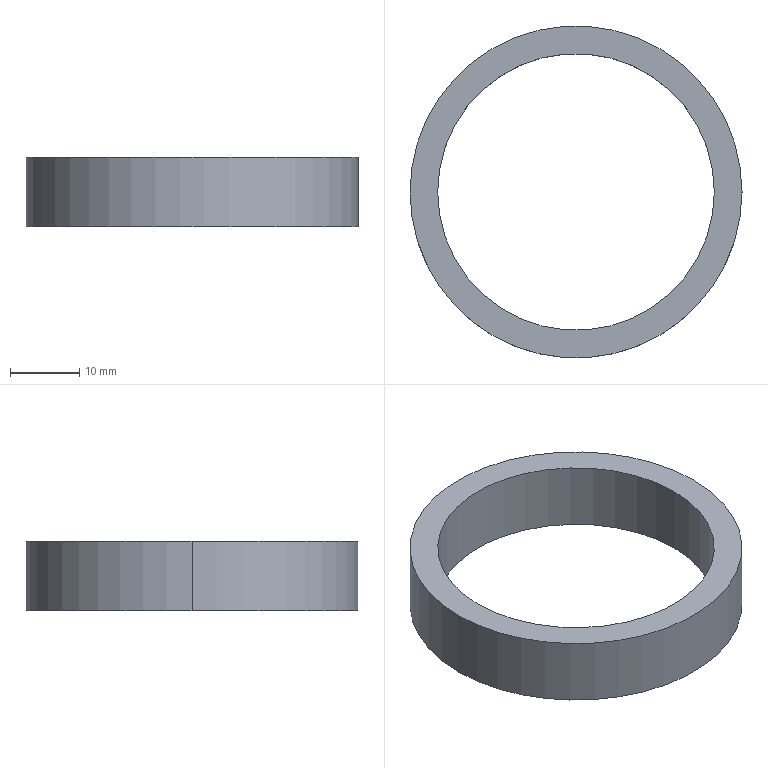Part | SolidWorks | features Extrusion 1 | 1 solid | 6 faces | box 48 x 48 x 10 mm | volume 5529 mm3 | cylinder 4 | plane 2 | commonest cylinder face diameters 40 x2 48 x2
STEP:
#1=CARTESIAN_POINT('',(-20.,0.,10.));
#2=VERTEX_POINT('',#1);
#3=CARTESIAN_POINT('',(20.,0.,10.));
#4=VERTEX_POINT('',#3);
#5=CARTESIAN_POINT('',(0.,0.,10.));
#6=DIRECTION('',(0.,0.,1.));
#7=DIRECTION('',(1.,0.,0.));
#8=AXIS2_PLACEMENT_3D('',#5,#6,#7);
#9=CIRCLE('',#8,20.);
#10=EDGE_CURVE('',#2,#4,#9,.T.);
#11=ORIENTED_EDGE('',*,*,#10,.T.);
#12=CARTESIAN_POINT('',(20.,0.,0.));
#13=VERTEX_POINT('',#12);
#14=CARTESIAN_POINT('',(20.,0.,10.));
#15=DIRECTION('',(0.,0.,-1.));
#16=VECTOR('',#15,1000.);
#17=LINE('',#14,#16);
#18=EDGE_CURVE('',#4,#13,#17,.T.);
#19=ORIENTED_EDGE('',*,*,#18,.T.);
#20=CARTESIAN_POINT('',(-20.,0.,0.));
#21=VERTEX_POINT('',#20);
#22=CARTESIAN_POINT('',(0.,0.,0.));
#23=DIRECTION('',(0.,0.,1.));
#24=DIRECTION('',(1.,0.,0.));
#25=AXIS2_PLACEMENT_3D('',#22,#23,#24);
#26=CIRCLE('',#25,20.);
#27=EDGE_CURVE('',#21,#13,#26,.T.);
#28=ORIENTED_EDGE('',*,*,#27,.F.);
#29=CARTESIAN_POINT('',(-20.,0.,10.));
#30=DIRECTION('',(0.,0.,-1.));
#31=VECTOR('',#30,1000.);
#32=LINE('',#29,#31);
#33=EDGE_CURVE('',#2,#21,#32,.T.);
#34=ORIENTED_EDGE('',*,*,#33,.F.);
#35=EDGE_LOOP('',(#11,#19,#28,#34));
#36=FACE_OUTER_BOUND('',#35,.T.);
#37=CARTESIAN_POINT('',(0.,0.,10.));
#38=DIRECTION('',(0.,0.,-1.));
#39=DIRECTION('',(-1.,0.,0.));
#40=AXIS2_PLACEMENT_3D('',#37,#38,#39);
#41=CYLINDRICAL_SURFACE('',#40,20.);
#42=ADVANCED_FACE('',(#36),#41,.F.);
#43=CARTESIAN_POINT('',(24.,0.,10.));
#44=VERTEX_POINT('',#43);
#45=CARTESIAN_POINT('',(-24.,0.,10.));
#46=VERTEX_POINT('',#45);
#47=CARTESIAN_POINT('',(0.,0.,10.));
#48=DIRECTION('',(0.,0.,1.));
#49=DIRECTION('',(1.,0.,0.));
#50=AXIS2_PLACEMENT_3D('',#47,#48,#49);
#51=CIRCLE('',#50,24.);
#52=EDGE_CURVE('',#44,#46,#51,.T.);
#53=ORIENTED_EDGE('',*,*,#52,.F.);
#54=CARTESIAN_POINT('',(24.,0.,0.));
#55=VERTEX_POINT('',#54);
#56=CARTESIAN_POINT('',(24.,0.,10.));
#57=DIRECTION('',(0.,0.,-1.));
#58=VECTOR('',#57,1000.);
#59=LINE('',#56,#58);
#60=EDGE_CURVE('',#44,#55,#59,.T.);
#61=ORIENTED_EDGE('',*,*,#60,.T.);
#62=CARTESIAN_POINT('',(-24.,0.,0.));
#63=VERTEX_POINT('',#62);
#64=CARTESIAN_POINT('',(0.,0.,0.));
#65=DIRECTION('',(0.,0.,1.));
#66=DIRECTION('',(1.,0.,0.));
#67=AXIS2_PLACEMENT_3D('',#64,#65,#66);
#68=CIRCLE('',#67,24.);
#69=EDGE_CURVE('',#55,#63,#68,.T.);
#70=ORIENTED_EDGE('',*,*,#69,.T.);
#71=CARTESIAN_POINT('',(-24.,0.,10.));
#72=DIRECTION('',(0.,0.,-1.));
#73=VECTOR('',#72,1000.);
#74=LINE('',#71,#73);
#75=EDGE_CURVE('',#46,#63,#74,.T.);
#76=ORIENTED_EDGE('',*,*,#75,.F.);
#77=EDGE_LOOP('',(#53,#61,#70,#76));
#78=FACE_OUTER_BOUND('',#77,.T.);
#79=CARTESIAN_POINT('',(0.,0.,10.));
#80=DIRECTION('',(0.,0.,-1.));
#81=DIRECTION('',(-1.,0.,0.));
#82=AXIS2_PLACEMENT_3D('',#79,#80,#81);
#83=CYLINDRICAL_SURFACE('',#82,24.);
#84=ADVANCED_FACE('',(#78),#83,.T.);
#85=CARTESIAN_POINT('',(0.,0.,10.));
#86=DIRECTION('',(0.,0.,1.));
#87=DIRECTION('',(1.,0.,0.));
#88=AXIS2_PLACEMENT_3D('',#85,#86,#87);
#89=CIRCLE('',#88,24.);
#90=EDGE_CURVE('',#46,#44,#89,.T.);
#91=ORIENTED_EDGE('',*,*,#90,.T.);
#92=ORIENTED_EDGE('',*,*,#52,.T.);
#93=EDGE_LOOP('',(#91,#92));
#94=FACE_OUTER_BOUND('',#93,.T.);
#95=ORIENTED_EDGE('',*,*,#10,.F.);
#96=CARTESIAN_POINT('',(0.,0.,10.));
#97=DIRECTION('',(0.,0.,1.));
#98=DIRECTION('',(1.,0.,0.));
#99=AXIS2_PLACEMENT_3D('',#96,#97,#98);
#100=CIRCLE('',#99,20.);
#101=EDGE_CURVE('',#4,#2,#100,.T.);
#102=ORIENTED_EDGE('',*,*,#101,.F.);
#103=EDGE_LOOP('',(#95,#102));
#104=FACE_BOUND('',#103,.T.);
#105=CARTESIAN_POINT('',(0.,0.,10.));
#106=DIRECTION('',(0.,0.,1.));
#107=DIRECTION('',(1.,0.,0.));
#108=AXIS2_PLACEMENT_3D('',#105,#106,#107);
#109=PLANE('',#108);
#110=ADVANCED_FACE('',(#94,#104),#109,.T.);
#111=CARTESIAN_POINT('',(0.,0.,0.));
#112=DIRECTION('',(0.,0.,1.));
#113=DIRECTION('',(1.,0.,0.));
#114=AXIS2_PLACEMENT_3D('',#111,#112,#113);
#115=CIRCLE('',#114,24.);
#116=EDGE_CURVE('',#63,#55,#115,.T.);
#117=ORIENTED_EDGE('',*,*,#116,.F.);
#118=ORIENTED_EDGE('',*,*,#69,.F.);
#119=EDGE_LOOP('',(#117,#118));
#120=FACE_OUTER_BOUND('',#119,.T.);
#121=ORIENTED_EDGE('',*,*,#27,.T.);
#122=CARTESIAN_POINT('',(0.,0.,0.));
#123=DIRECTION('',(0.,0.,1.));
#124=DIRECTION('',(1.,0.,0.));
#125=AXIS2_PLACEMENT_3D('',#122,#123,#124);
#126=CIRCLE('',#125,20.);
#127=EDGE_CURVE('',#13,#21,#126,.T.);
#128=ORIENTED_EDGE('',*,*,#127,.T.);
#129=EDGE_LOOP('',(#121,#128));
#130=FACE_BOUND('',#129,.T.);
#131=CARTESIAN_POINT('',(0.,0.,0.));
#132=DIRECTION('',(0.,0.,1.));
#133=DIRECTION('',(1.,0.,0.));
#134=AXIS2_PLACEMENT_3D('',#131,#132,#133);
#135=PLANE('',#134);
#136=ADVANCED_FACE('',(#120,#130),#135,.F.);
#137=ORIENTED_EDGE('',*,*,#60,.F.);
#138=ORIENTED_EDGE('',*,*,#90,.F.);
#139=ORIENTED_EDGE('',*,*,#75,.T.);
#140=ORIENTED_EDGE('',*,*,#116,.T.);
#141=EDGE_LOOP('',(#137,#138,#139,#140));
#142=FACE_OUTER_BOUND('',#141,.T.);
#143=CARTESIAN_POINT('',(0.,0.,10.));
#144=DIRECTION('',(0.,0.,-1.));
#145=DIRECTION('',(-1.,0.,0.));
#146=AXIS2_PLACEMENT_3D('',#143,#144,#145);
#147=CYLINDRICAL_SURFACE('',#146,24.);
#148=ADVANCED_FACE('',(#142),#147,.T.);
#149=ORIENTED_EDGE('',*,*,#18,.F.);
#150=ORIENTED_EDGE('',*,*,#101,.T.);
#151=ORIENTED_EDGE('',*,*,#33,.T.);
#152=ORIENTED_EDGE('',*,*,#127,.F.);
#153=EDGE_LOOP('',(#149,#150,#151,#152));
#154=FACE_OUTER_BOUND('',#153,.T.);
#155=CARTESIAN_POINT('',(0.,0.,10.));
#156=DIRECTION('',(0.,0.,-1.));
#157=DIRECTION('',(-1.,0.,0.));
#158=AXIS2_PLACEMENT_3D('',#155,#156,#157);
#159=CYLINDRICAL_SURFACE('',#158,20.);
#160=ADVANCED_FACE('',(#154),#159,.F.);
#161=CLOSED_SHELL('',(#42,#84,#110,#136,#148,#160));
#162=MANIFOLD_SOLID_BREP('',#161);
#163=CARTESIAN_POINT('',(0.,0.,0.));
#164=DIRECTION('',(0.,0.,1.));
#165=DIRECTION('',(1.,0.,0.));
#166=AXIS2_PLACEMENT_3D('',#163,#164,#165);
#167=(LENGTH_UNIT()NAMED_UNIT(*)SI_UNIT(.MILLI.,.METRE.));
#168=UNCERTAINTY_MEASURE_WITH_UNIT(LENGTH_MEASURE(0.00001),#167,'','');
#169=(NAMED_UNIT(*)PLANE_ANGLE_UNIT()SI_UNIT($,.RADIAN.));
#170=(NAMED_UNIT(*)SI_UNIT($,.STERADIAN.)SOLID_ANGLE_UNIT());
#171=(GEOMETRIC_REPRESENTATION_CONTEXT(3)GLOBAL_UNCERTAINTY_ASSIGNED_CONTEXT((#168))GLOBAL_UNIT_ASSIGNED_CONTEXT((#167,#169,#170))REPRESENTATION_CONTEXT('',''));
#172=ADVANCED_BREP_SHAPE_REPRESENTATION('',(#162,#166),#171);